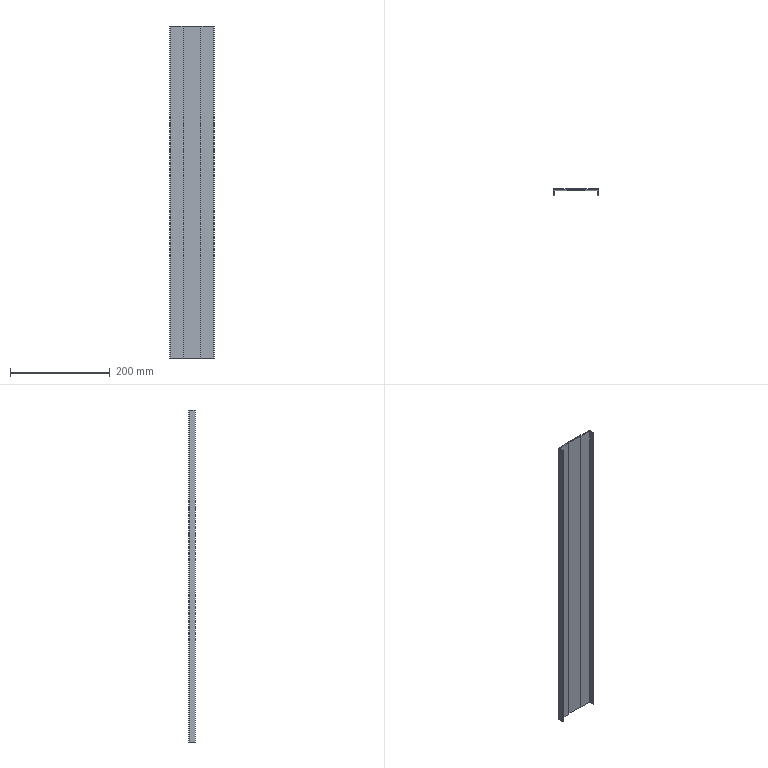Part | NX | 1 solid | 18 faces | box 89 x 13 x 666 mm | volume 147852 mm3 | plane 18
STEP:
#1=CARTESIAN_POINT('',(42.5,10.,-333.));
#2=VERTEX_POINT('',#1);
#3=CARTESIAN_POINT('',(42.5,0.,-333.));
#4=VERTEX_POINT('',#3);
#5=CARTESIAN_POINT('',(42.5,12.,-333.));
#6=DIRECTION('',(0.,-1.,0.));
#7=VECTOR('',#6,1000.);
#8=LINE('',#5,#7);
#9=EDGE_CURVE('',#2,#4,#8,.T.);
#10=ORIENTED_EDGE('',*,*,#9,.T.);
#11=CARTESIAN_POINT('',(42.5,0.,333.));
#12=VERTEX_POINT('',#11);
#13=CARTESIAN_POINT('',(42.5,0.,333.));
#14=DIRECTION('',(0.,0.,-1.));
#15=VECTOR('',#14,1000.);
#16=LINE('',#13,#15);
#17=EDGE_CURVE('',#12,#4,#16,.T.);
#18=ORIENTED_EDGE('',*,*,#17,.F.);
#19=CARTESIAN_POINT('',(42.5,10.,333.));
#20=VERTEX_POINT('',#19);
#21=CARTESIAN_POINT('',(42.5,12.,333.));
#22=DIRECTION('',(0.,-1.,0.));
#23=VECTOR('',#22,1000.);
#24=LINE('',#21,#23);
#25=EDGE_CURVE('',#20,#12,#24,.T.);
#26=ORIENTED_EDGE('',*,*,#25,.F.);
#27=CARTESIAN_POINT('',(42.5,10.,333.));
#28=DIRECTION('',(0.,0.,-1.));
#29=VECTOR('',#28,1000.);
#30=LINE('',#27,#29);
#31=EDGE_CURVE('',#20,#2,#30,.T.);
#32=ORIENTED_EDGE('',*,*,#31,.T.);
#33=EDGE_LOOP('',(#10,#18,#26,#32));
#34=FACE_BOUND('',#33,.T.);
#35=CARTESIAN_POINT('',(42.5,12.,333.));
#36=DIRECTION('',(1.,0.,0.));
#37=DIRECTION('',(0.,1.,0.));
#38=AXIS2_PLACEMENT_3D('',#35,#36,#37);
#39=PLANE('',#38);
#40=ADVANCED_FACE('',(#34),#39,.F.);
#41=CARTESIAN_POINT('',(44.5,0.,-333.));
#42=VERTEX_POINT('',#41);
#43=CARTESIAN_POINT('',(44.5,0.,-333.));
#44=DIRECTION('',(-1.,0.,0.));
#45=VECTOR('',#44,1000.);
#46=LINE('',#43,#45);
#47=EDGE_CURVE('',#42,#4,#46,.T.);
#48=ORIENTED_EDGE('',*,*,#47,.F.);
#49=CARTESIAN_POINT('',(44.5,0.,333.));
#50=VERTEX_POINT('',#49);
#51=CARTESIAN_POINT('',(44.5,0.,333.));
#52=DIRECTION('',(0.,0.,-1.));
#53=VECTOR('',#52,1000.);
#54=LINE('',#51,#53);
#55=EDGE_CURVE('',#50,#42,#54,.T.);
#56=ORIENTED_EDGE('',*,*,#55,.F.);
#57=CARTESIAN_POINT('',(44.5,0.,333.));
#58=DIRECTION('',(-1.,0.,0.));
#59=VECTOR('',#58,1000.);
#60=LINE('',#57,#59);
#61=EDGE_CURVE('',#50,#12,#60,.T.);
#62=ORIENTED_EDGE('',*,*,#61,.T.);
#63=ORIENTED_EDGE('',*,*,#17,.T.);
#64=EDGE_LOOP('',(#48,#56,#62,#63));
#65=FACE_BOUND('',#64,.T.);
#66=CARTESIAN_POINT('',(44.5,0.,333.));
#67=DIRECTION('',(0.,-1.,0.));
#68=DIRECTION('',(1.,0.,0.));
#69=AXIS2_PLACEMENT_3D('',#66,#67,#68);
#70=PLANE('',#69);
#71=ADVANCED_FACE('',(#65),#70,.T.);
#72=CARTESIAN_POINT('',(44.5,12.,-333.));
#73=VERTEX_POINT('',#72);
#74=CARTESIAN_POINT('',(44.5,12.,-333.));
#75=DIRECTION('',(0.,-1.,0.));
#76=VECTOR('',#75,1000.);
#77=LINE('',#74,#76);
#78=EDGE_CURVE('',#73,#42,#77,.T.);
#79=ORIENTED_EDGE('',*,*,#78,.F.);
#80=CARTESIAN_POINT('',(44.5,12.,333.));
#81=VERTEX_POINT('',#80);
#82=CARTESIAN_POINT('',(44.5,12.,333.));
#83=DIRECTION('',(0.,0.,-1.));
#84=VECTOR('',#83,1000.);
#85=LINE('',#82,#84);
#86=EDGE_CURVE('',#81,#73,#85,.T.);
#87=ORIENTED_EDGE('',*,*,#86,.F.);
#88=CARTESIAN_POINT('',(44.5,12.,333.));
#89=DIRECTION('',(0.,-1.,0.));
#90=VECTOR('',#89,1000.);
#91=LINE('',#88,#90);
#92=EDGE_CURVE('',#81,#50,#91,.T.);
#93=ORIENTED_EDGE('',*,*,#92,.T.);
#94=ORIENTED_EDGE('',*,*,#55,.T.);
#95=EDGE_LOOP('',(#79,#87,#93,#94));
#96=FACE_BOUND('',#95,.T.);
#97=CARTESIAN_POINT('',(44.5,12.,333.));
#98=DIRECTION('',(1.,0.,0.));
#99=DIRECTION('',(0.,1.,0.));
#100=AXIS2_PLACEMENT_3D('',#97,#98,#99);
#101=PLANE('',#100);
#102=ADVANCED_FACE('',(#96),#101,.T.);
#103=CARTESIAN_POINT('',(20.,12.,-333.));
#104=VERTEX_POINT('',#103);
#105=CARTESIAN_POINT('',(20.,12.,-333.));
#106=DIRECTION('',(1.,0.,0.));
#107=VECTOR('',#106,1000.);
#108=LINE('',#105,#107);
#109=EDGE_CURVE('',#104,#73,#108,.T.);
#110=ORIENTED_EDGE('',*,*,#109,.F.);
#111=CARTESIAN_POINT('',(20.,12.,333.));
#112=VERTEX_POINT('',#111);
#113=CARTESIAN_POINT('',(20.,12.,333.));
#114=DIRECTION('',(0.,0.,-1.));
#115=VECTOR('',#114,1000.);
#116=LINE('',#113,#115);
#117=EDGE_CURVE('',#112,#104,#116,.T.);
#118=ORIENTED_EDGE('',*,*,#117,.F.);
#119=CARTESIAN_POINT('',(20.,12.,333.));
#120=DIRECTION('',(1.,0.,0.));
#121=VECTOR('',#120,1000.);
#122=LINE('',#119,#121);
#123=EDGE_CURVE('',#112,#81,#122,.T.);
#124=ORIENTED_EDGE('',*,*,#123,.T.);
#125=ORIENTED_EDGE('',*,*,#86,.T.);
#126=EDGE_LOOP('',(#110,#118,#124,#125));
#127=FACE_BOUND('',#126,.T.);
#128=CARTESIAN_POINT('',(20.,12.,333.));
#129=DIRECTION('',(0.,1.,0.));
#130=DIRECTION('',(-1.,0.,0.));
#131=AXIS2_PLACEMENT_3D('',#128,#129,#130);
#132=PLANE('',#131);
#133=ADVANCED_FACE('',(#127),#132,.T.);
#134=CARTESIAN_POINT('',(20.,13.,-333.));
#135=VERTEX_POINT('',#134);
#136=CARTESIAN_POINT('',(20.,13.,-333.));
#137=DIRECTION('',(0.,-1.,0.));
#138=VECTOR('',#137,1000.);
#139=LINE('',#136,#138);
#140=EDGE_CURVE('',#135,#104,#139,.T.);
#141=ORIENTED_EDGE('',*,*,#140,.F.);
#142=CARTESIAN_POINT('',(20.,13.,333.));
#143=VERTEX_POINT('',#142);
#144=CARTESIAN_POINT('',(20.,13.,333.));
#145=DIRECTION('',(0.,0.,-1.));
#146=VECTOR('',#145,1000.);
#147=LINE('',#144,#146);
#148=EDGE_CURVE('',#143,#135,#147,.T.);
#149=ORIENTED_EDGE('',*,*,#148,.F.);
#150=CARTESIAN_POINT('',(20.,13.,333.));
#151=DIRECTION('',(0.,-1.,0.));
#152=VECTOR('',#151,1000.);
#153=LINE('',#150,#152);
#154=EDGE_CURVE('',#143,#112,#153,.T.);
#155=ORIENTED_EDGE('',*,*,#154,.T.);
#156=ORIENTED_EDGE('',*,*,#117,.T.);
#157=EDGE_LOOP('',(#141,#149,#155,#156));
#158=FACE_BOUND('',#157,.T.);
#159=CARTESIAN_POINT('',(20.,13.,333.));
#160=DIRECTION('',(1.,0.,0.));
#161=DIRECTION('',(0.,0.,-1.));
#162=AXIS2_PLACEMENT_3D('',#159,#160,#161);
#163=PLANE('',#162);
#164=ADVANCED_FACE('',(#158),#163,.T.);
#165=CARTESIAN_POINT('',(-20.,13.,-333.));
#166=VERTEX_POINT('',#165);
#167=CARTESIAN_POINT('',(-20.,13.,-333.));
#168=DIRECTION('',(1.,0.,0.));
#169=VECTOR('',#168,1000.);
#170=LINE('',#167,#169);
#171=EDGE_CURVE('',#166,#135,#170,.T.);
#172=ORIENTED_EDGE('',*,*,#171,.F.);
#173=CARTESIAN_POINT('',(-20.,13.,333.));
#174=VERTEX_POINT('',#173);
#175=CARTESIAN_POINT('',(-20.,13.,333.));
#176=DIRECTION('',(0.,0.,-1.));
#177=VECTOR('',#176,1000.);
#178=LINE('',#175,#177);
#179=EDGE_CURVE('',#174,#166,#178,.T.);
#180=ORIENTED_EDGE('',*,*,#179,.F.);
#181=CARTESIAN_POINT('',(-20.,13.,333.));
#182=DIRECTION('',(1.,0.,0.));
#183=VECTOR('',#182,1000.);
#184=LINE('',#181,#183);
#185=EDGE_CURVE('',#174,#143,#184,.T.);
#186=ORIENTED_EDGE('',*,*,#185,.T.);
#187=ORIENTED_EDGE('',*,*,#148,.T.);
#188=EDGE_LOOP('',(#172,#180,#186,#187));
#189=FACE_BOUND('',#188,.T.);
#190=CARTESIAN_POINT('',(-20.,13.,333.));
#191=DIRECTION('',(0.,1.,0.));
#192=DIRECTION('',(-1.,0.,0.));
#193=AXIS2_PLACEMENT_3D('',#190,#191,#192);
#194=PLANE('',#193);
#195=ADVANCED_FACE('',(#189),#194,.T.);
#196=CARTESIAN_POINT('',(-20.,12.,-333.));
#197=VERTEX_POINT('',#196);
#198=CARTESIAN_POINT('',(-20.,12.,-333.));
#199=DIRECTION('',(0.,1.,0.));
#200=VECTOR('',#199,1000.);
#201=LINE('',#198,#200);
#202=EDGE_CURVE('',#197,#166,#201,.T.);
#203=ORIENTED_EDGE('',*,*,#202,.F.);
#204=CARTESIAN_POINT('',(-20.,12.,333.));
#205=VERTEX_POINT('',#204);
#206=CARTESIAN_POINT('',(-20.,12.,333.));
#207=DIRECTION('',(0.,0.,-1.));
#208=VECTOR('',#207,1000.);
#209=LINE('',#206,#208);
#210=EDGE_CURVE('',#205,#197,#209,.T.);
#211=ORIENTED_EDGE('',*,*,#210,.F.);
#212=CARTESIAN_POINT('',(-20.,12.,333.));
#213=DIRECTION('',(0.,1.,0.));
#214=VECTOR('',#213,1000.);
#215=LINE('',#212,#214);
#216=EDGE_CURVE('',#205,#174,#215,.T.);
#217=ORIENTED_EDGE('',*,*,#216,.T.);
#218=ORIENTED_EDGE('',*,*,#179,.T.);
#219=EDGE_LOOP('',(#203,#211,#217,#218));
#220=FACE_BOUND('',#219,.T.);
#221=CARTESIAN_POINT('',(-20.,12.,333.));
#222=DIRECTION('',(-1.,0.,0.));
#223=DIRECTION('',(0.,0.,1.));
#224=AXIS2_PLACEMENT_3D('',#221,#222,#223);
#225=PLANE('',#224);
#226=ADVANCED_FACE('',(#220),#225,.T.);
#227=CARTESIAN_POINT('',(-44.5,12.,-333.));
#228=VERTEX_POINT('',#227);
#229=CARTESIAN_POINT('',(-44.5,12.,-333.));
#230=DIRECTION('',(1.,0.,0.));
#231=VECTOR('',#230,1000.);
#232=LINE('',#229,#231);
#233=EDGE_CURVE('',#228,#197,#232,.T.);
#234=ORIENTED_EDGE('',*,*,#233,.F.);
#235=CARTESIAN_POINT('',(-44.5,12.,333.));
#236=VERTEX_POINT('',#235);
#237=CARTESIAN_POINT('',(-44.5,12.,333.));
#238=DIRECTION('',(0.,0.,-1.));
#239=VECTOR('',#238,1000.);
#240=LINE('',#237,#239);
#241=EDGE_CURVE('',#236,#228,#240,.T.);
#242=ORIENTED_EDGE('',*,*,#241,.F.);
#243=CARTESIAN_POINT('',(-44.5,12.,333.));
#244=DIRECTION('',(1.,0.,0.));
#245=VECTOR('',#244,1000.);
#246=LINE('',#243,#245);
#247=EDGE_CURVE('',#236,#205,#246,.T.);
#248=ORIENTED_EDGE('',*,*,#247,.T.);
#249=ORIENTED_EDGE('',*,*,#210,.T.);
#250=EDGE_LOOP('',(#234,#242,#248,#249));
#251=FACE_BOUND('',#250,.T.);
#252=CARTESIAN_POINT('',(-44.5,12.,333.));
#253=DIRECTION('',(0.,1.,0.));
#254=DIRECTION('',(0.,0.,1.));
#255=AXIS2_PLACEMENT_3D('',#252,#253,#254);
#256=PLANE('',#255);
#257=ADVANCED_FACE('',(#251),#256,.T.);
#258=CARTESIAN_POINT('',(-44.5,0.,-333.));
#259=VERTEX_POINT('',#258);
#260=CARTESIAN_POINT('',(-44.5,0.,-333.));
#261=DIRECTION('',(0.,1.,0.));
#262=VECTOR('',#261,1000.);
#263=LINE('',#260,#262);
#264=EDGE_CURVE('',#259,#228,#263,.T.);
#265=ORIENTED_EDGE('',*,*,#264,.F.);
#266=CARTESIAN_POINT('',(-44.5,0.,333.));
#267=VERTEX_POINT('',#266);
#268=CARTESIAN_POINT('',(-44.5,0.,333.));
#269=DIRECTION('',(0.,0.,-1.));
#270=VECTOR('',#269,1000.);
#271=LINE('',#268,#270);
#272=EDGE_CURVE('',#267,#259,#271,.T.);
#273=ORIENTED_EDGE('',*,*,#272,.F.);
#274=CARTESIAN_POINT('',(-44.5,0.,333.));
#275=DIRECTION('',(0.,1.,0.));
#276=VECTOR('',#275,1000.);
#277=LINE('',#274,#276);
#278=EDGE_CURVE('',#267,#236,#277,.T.);
#279=ORIENTED_EDGE('',*,*,#278,.T.);
#280=ORIENTED_EDGE('',*,*,#241,.T.);
#281=EDGE_LOOP('',(#265,#273,#279,#280));
#282=FACE_BOUND('',#281,.T.);
#283=CARTESIAN_POINT('',(-44.5,0.,333.));
#284=DIRECTION('',(-1.,0.,0.));
#285=DIRECTION('',(0.,0.,1.));
#286=AXIS2_PLACEMENT_3D('',#283,#284,#285);
#287=PLANE('',#286);
#288=ADVANCED_FACE('',(#282),#287,.T.);
#289=CARTESIAN_POINT('',(-42.5,0.,-333.));
#290=VERTEX_POINT('',#289);
#291=CARTESIAN_POINT('',(-42.5,0.,-333.));
#292=DIRECTION('',(-1.,0.,0.));
#293=VECTOR('',#292,1000.);
#294=LINE('',#291,#293);
#295=EDGE_CURVE('',#290,#259,#294,.T.);
#296=ORIENTED_EDGE('',*,*,#295,.F.);
#297=CARTESIAN_POINT('',(-42.5,0.,333.));
#298=VERTEX_POINT('',#297);
#299=CARTESIAN_POINT('',(-42.5,0.,333.));
#300=DIRECTION('',(0.,0.,-1.));
#301=VECTOR('',#300,1000.);
#302=LINE('',#299,#301);
#303=EDGE_CURVE('',#298,#290,#302,.T.);
#304=ORIENTED_EDGE('',*,*,#303,.F.);
#305=CARTESIAN_POINT('',(-42.5,0.,333.));
#306=DIRECTION('',(-1.,0.,0.));
#307=VECTOR('',#306,1000.);
#308=LINE('',#305,#307);
#309=EDGE_CURVE('',#298,#267,#308,.T.);
#310=ORIENTED_EDGE('',*,*,#309,.T.);
#311=ORIENTED_EDGE('',*,*,#272,.T.);
#312=EDGE_LOOP('',(#296,#304,#310,#311));
#313=FACE_BOUND('',#312,.T.);
#314=CARTESIAN_POINT('',(-42.5,0.,333.));
#315=DIRECTION('',(0.,-1.,0.));
#316=DIRECTION('',(0.,0.,-1.));
#317=AXIS2_PLACEMENT_3D('',#314,#315,#316);
#318=PLANE('',#317);
#319=ADVANCED_FACE('',(#313),#318,.T.);
#320=CARTESIAN_POINT('',(-42.5,10.,-333.));
#321=VERTEX_POINT('',#320);
#322=CARTESIAN_POINT('',(-42.5,0.,-333.));
#323=DIRECTION('',(0.,1.,0.));
#324=VECTOR('',#323,1000.);
#325=LINE('',#322,#324);
#326=EDGE_CURVE('',#290,#321,#325,.T.);
#327=ORIENTED_EDGE('',*,*,#326,.T.);
#328=CARTESIAN_POINT('',(-42.5,10.,333.));
#329=VERTEX_POINT('',#328);
#330=CARTESIAN_POINT('',(-42.5,10.,333.));
#331=DIRECTION('',(0.,0.,-1.));
#332=VECTOR('',#331,1000.);
#333=LINE('',#330,#332);
#334=EDGE_CURVE('',#329,#321,#333,.T.);
#335=ORIENTED_EDGE('',*,*,#334,.F.);
#336=CARTESIAN_POINT('',(-42.5,0.,333.));
#337=DIRECTION('',(0.,1.,0.));
#338=VECTOR('',#337,1000.);
#339=LINE('',#336,#338);
#340=EDGE_CURVE('',#298,#329,#339,.T.);
#341=ORIENTED_EDGE('',*,*,#340,.F.);
#342=ORIENTED_EDGE('',*,*,#303,.T.);
#343=EDGE_LOOP('',(#327,#335,#341,#342));
#344=FACE_BOUND('',#343,.T.);
#345=CARTESIAN_POINT('',(-42.5,0.,333.));
#346=DIRECTION('',(-1.,0.,0.));
#347=DIRECTION('',(0.,0.,1.));
#348=AXIS2_PLACEMENT_3D('',#345,#346,#347);
#349=PLANE('',#348);
#350=ADVANCED_FACE('',(#344),#349,.F.);
#351=CARTESIAN_POINT('',(-18.,10.,-333.));
#352=VERTEX_POINT('',#351);
#353=CARTESIAN_POINT('',(-44.5,10.,-333.));
#354=DIRECTION('',(1.,0.,0.));
#355=VECTOR('',#354,1000.);
#356=LINE('',#353,#355);
#357=EDGE_CURVE('',#321,#352,#356,.T.);
#358=ORIENTED_EDGE('',*,*,#357,.T.);
#359=CARTESIAN_POINT('',(-18.,10.,333.));
#360=VERTEX_POINT('',#359);
#361=CARTESIAN_POINT('',(-18.,10.,333.));
#362=DIRECTION('',(0.,0.,-1.));
#363=VECTOR('',#362,1000.);
#364=LINE('',#361,#363);
#365=EDGE_CURVE('',#360,#352,#364,.T.);
#366=ORIENTED_EDGE('',*,*,#365,.F.);
#367=CARTESIAN_POINT('',(-44.5,10.,333.));
#368=DIRECTION('',(1.,0.,0.));
#369=VECTOR('',#368,1000.);
#370=LINE('',#367,#369);
#371=EDGE_CURVE('',#329,#360,#370,.T.);
#372=ORIENTED_EDGE('',*,*,#371,.F.);
#373=ORIENTED_EDGE('',*,*,#334,.T.);
#374=EDGE_LOOP('',(#358,#366,#372,#373));
#375=FACE_BOUND('',#374,.T.);
#376=CARTESIAN_POINT('',(-44.5,10.,333.));
#377=DIRECTION('',(0.,1.,0.));
#378=DIRECTION('',(0.,0.,1.));
#379=AXIS2_PLACEMENT_3D('',#376,#377,#378);
#380=PLANE('',#379);
#381=ADVANCED_FACE('',(#375),#380,.F.);
#382=CARTESIAN_POINT('',(-18.,11.,-333.));
#383=VERTEX_POINT('',#382);
#384=CARTESIAN_POINT('',(-18.,12.,-333.));
#385=DIRECTION('',(0.,1.,0.));
#386=VECTOR('',#385,1000.);
#387=LINE('',#384,#386);
#388=EDGE_CURVE('',#352,#383,#387,.T.);
#389=ORIENTED_EDGE('',*,*,#388,.T.);
#390=CARTESIAN_POINT('',(-18.,11.,333.));
#391=VERTEX_POINT('',#390);
#392=CARTESIAN_POINT('',(-18.,11.,333.));
#393=DIRECTION('',(0.,0.,-1.));
#394=VECTOR('',#393,1000.);
#395=LINE('',#392,#394);
#396=EDGE_CURVE('',#391,#383,#395,.T.);
#397=ORIENTED_EDGE('',*,*,#396,.F.);
#398=CARTESIAN_POINT('',(-18.,12.,333.));
#399=DIRECTION('',(0.,1.,0.));
#400=VECTOR('',#399,1000.);
#401=LINE('',#398,#400);
#402=EDGE_CURVE('',#360,#391,#401,.T.);
#403=ORIENTED_EDGE('',*,*,#402,.F.);
#404=ORIENTED_EDGE('',*,*,#365,.T.);
#405=EDGE_LOOP('',(#389,#397,#403,#404));
#406=FACE_BOUND('',#405,.T.);
#407=CARTESIAN_POINT('',(-18.,12.,333.));
#408=DIRECTION('',(-1.,0.,0.));
#409=DIRECTION('',(0.,0.,1.));
#410=AXIS2_PLACEMENT_3D('',#407,#408,#409);
#411=PLANE('',#410);
#412=ADVANCED_FACE('',(#406),#411,.F.);
#413=CARTESIAN_POINT('',(18.,11.,-333.));
#414=VERTEX_POINT('',#413);
#415=CARTESIAN_POINT('',(-20.,11.,-333.));
#416=DIRECTION('',(1.,0.,0.));
#417=VECTOR('',#416,1000.);
#418=LINE('',#415,#417);
#419=EDGE_CURVE('',#383,#414,#418,.T.);
#420=ORIENTED_EDGE('',*,*,#419,.T.);
#421=CARTESIAN_POINT('',(18.,11.,333.));
#422=VERTEX_POINT('',#421);
#423=CARTESIAN_POINT('',(18.,11.,333.));
#424=DIRECTION('',(0.,0.,-1.));
#425=VECTOR('',#424,1000.);
#426=LINE('',#423,#425);
#427=EDGE_CURVE('',#422,#414,#426,.T.);
#428=ORIENTED_EDGE('',*,*,#427,.F.);
#429=CARTESIAN_POINT('',(-20.,11.,333.));
#430=DIRECTION('',(1.,0.,0.));
#431=VECTOR('',#430,1000.);
#432=LINE('',#429,#431);
#433=EDGE_CURVE('',#391,#422,#432,.T.);
#434=ORIENTED_EDGE('',*,*,#433,.F.);
#435=ORIENTED_EDGE('',*,*,#396,.T.);
#436=EDGE_LOOP('',(#420,#428,#434,#435));
#437=FACE_BOUND('',#436,.T.);
#438=CARTESIAN_POINT('',(-20.,11.,333.));
#439=DIRECTION('',(0.,1.,0.));
#440=DIRECTION('',(-1.,0.,0.));
#441=AXIS2_PLACEMENT_3D('',#438,#439,#440);
#442=PLANE('',#441);
#443=ADVANCED_FACE('',(#437),#442,.F.);
#444=CARTESIAN_POINT('',(18.,10.,-333.));
#445=VERTEX_POINT('',#444);
#446=CARTESIAN_POINT('',(18.,13.,-333.));
#447=DIRECTION('',(0.,1.,0.));
#448=VECTOR('',#447,1000.);
#449=LINE('',#446,#448);
#450=EDGE_CURVE('',#414,#445,#449,.F.);
#451=ORIENTED_EDGE('',*,*,#450,.T.);
#452=CARTESIAN_POINT('',(18.,10.,333.));
#453=VERTEX_POINT('',#452);
#454=CARTESIAN_POINT('',(18.,10.,333.));
#455=DIRECTION('',(0.,0.,-1.));
#456=VECTOR('',#455,1000.);
#457=LINE('',#454,#456);
#458=EDGE_CURVE('',#453,#445,#457,.T.);
#459=ORIENTED_EDGE('',*,*,#458,.F.);
#460=CARTESIAN_POINT('',(18.,13.,333.));
#461=DIRECTION('',(0.,1.,0.));
#462=VECTOR('',#461,1000.);
#463=LINE('',#460,#462);
#464=EDGE_CURVE('',#422,#453,#463,.F.);
#465=ORIENTED_EDGE('',*,*,#464,.F.);
#466=ORIENTED_EDGE('',*,*,#427,.T.);
#467=EDGE_LOOP('',(#451,#459,#465,#466));
#468=FACE_BOUND('',#467,.T.);
#469=CARTESIAN_POINT('',(18.,13.,333.));
#470=DIRECTION('',(1.,0.,0.));
#471=DIRECTION('',(0.,0.,-1.));
#472=AXIS2_PLACEMENT_3D('',#469,#470,#471);
#473=PLANE('',#472);
#474=ADVANCED_FACE('',(#468),#473,.F.);
#475=CARTESIAN_POINT('',(20.,10.,-333.));
#476=DIRECTION('',(1.,0.,0.));
#477=VECTOR('',#476,1000.);
#478=LINE('',#475,#477);
#479=EDGE_CURVE('',#445,#2,#478,.T.);
#480=ORIENTED_EDGE('',*,*,#479,.T.);
#481=ORIENTED_EDGE('',*,*,#31,.F.);
#482=CARTESIAN_POINT('',(20.,10.,333.));
#483=DIRECTION('',(1.,0.,0.));
#484=VECTOR('',#483,1000.);
#485=LINE('',#482,#484);
#486=EDGE_CURVE('',#453,#20,#485,.T.);
#487=ORIENTED_EDGE('',*,*,#486,.F.);
#488=ORIENTED_EDGE('',*,*,#458,.T.);
#489=EDGE_LOOP('',(#480,#481,#487,#488));
#490=FACE_BOUND('',#489,.T.);
#491=CARTESIAN_POINT('',(20.,10.,333.));
#492=DIRECTION('',(0.,1.,0.));
#493=DIRECTION('',(-1.,0.,0.));
#494=AXIS2_PLACEMENT_3D('',#491,#492,#493);
#495=PLANE('',#494);
#496=ADVANCED_FACE('',(#490),#495,.F.);
#497=ORIENTED_EDGE('',*,*,#25,.T.);
#498=ORIENTED_EDGE('',*,*,#61,.F.);
#499=ORIENTED_EDGE('',*,*,#92,.F.);
#500=ORIENTED_EDGE('',*,*,#123,.F.);
#501=ORIENTED_EDGE('',*,*,#154,.F.);
#502=ORIENTED_EDGE('',*,*,#185,.F.);
#503=ORIENTED_EDGE('',*,*,#216,.F.);
#504=ORIENTED_EDGE('',*,*,#247,.F.);
#505=ORIENTED_EDGE('',*,*,#278,.F.);
#506=ORIENTED_EDGE('',*,*,#309,.F.);
#507=ORIENTED_EDGE('',*,*,#340,.T.);
#508=ORIENTED_EDGE('',*,*,#371,.T.);
#509=ORIENTED_EDGE('',*,*,#402,.T.);
#510=ORIENTED_EDGE('',*,*,#433,.T.);
#511=ORIENTED_EDGE('',*,*,#464,.T.);
#512=ORIENTED_EDGE('',*,*,#486,.T.);
#513=EDGE_LOOP('',(#497,#498,#499,#500,#501,#502,#503,#504,#505,#506,#507,#508,#509,#510,#511,#512));
#514=FACE_BOUND('',#513,.T.);
#515=CARTESIAN_POINT('',(0.,0.,333.));
#516=DIRECTION('',(0.,0.,-1.));
#517=DIRECTION('',(-1.,0.,0.));
#518=AXIS2_PLACEMENT_3D('',#515,#516,#517);
#519=PLANE('',#518);
#520=ADVANCED_FACE('',(#514),#519,.F.);
#521=ORIENTED_EDGE('',*,*,#9,.F.);
#522=ORIENTED_EDGE('',*,*,#479,.F.);
#523=ORIENTED_EDGE('',*,*,#450,.F.);
#524=ORIENTED_EDGE('',*,*,#419,.F.);
#525=ORIENTED_EDGE('',*,*,#388,.F.);
#526=ORIENTED_EDGE('',*,*,#357,.F.);
#527=ORIENTED_EDGE('',*,*,#326,.F.);
#528=ORIENTED_EDGE('',*,*,#295,.T.);
#529=ORIENTED_EDGE('',*,*,#264,.T.);
#530=ORIENTED_EDGE('',*,*,#233,.T.);
#531=ORIENTED_EDGE('',*,*,#202,.T.);
#532=ORIENTED_EDGE('',*,*,#171,.T.);
#533=ORIENTED_EDGE('',*,*,#140,.T.);
#534=ORIENTED_EDGE('',*,*,#109,.T.);
#535=ORIENTED_EDGE('',*,*,#78,.T.);
#536=ORIENTED_EDGE('',*,*,#47,.T.);
#537=EDGE_LOOP('',(#521,#522,#523,#524,#525,#526,#527,#528,#529,#530,#531,#532,#533,#534,#535,#536));
#538=FACE_BOUND('',#537,.T.);
#539=CARTESIAN_POINT('',(0.,0.,-333.));
#540=DIRECTION('',(0.,0.,-1.));
#541=DIRECTION('',(-1.,0.,0.));
#542=AXIS2_PLACEMENT_3D('',#539,#540,#541);
#543=PLANE('',#542);
#544=ADVANCED_FACE('',(#538),#543,.T.);
#545=CLOSED_SHELL('',(#40,#71,#102,#133,#164,#195,#226,#257,#288,#319,#350,#381,#412,#443,#474,#496,#520,#544));
#546=MANIFOLD_SOLID_BREP('',#545);
#547=(LENGTH_UNIT()NAMED_UNIT(*)SI_UNIT(.MILLI.,.METRE.));
#548=UNCERTAINTY_MEASURE_WITH_UNIT(LENGTH_MEASURE(0.00001),#547,'','');
#549=(NAMED_UNIT(*)PLANE_ANGLE_UNIT()SI_UNIT($,.RADIAN.));
#550=(NAMED_UNIT(*)SI_UNIT($,.STERADIAN.)SOLID_ANGLE_UNIT());
#551=(GEOMETRIC_REPRESENTATION_CONTEXT(3)GLOBAL_UNCERTAINTY_ASSIGNED_CONTEXT((#548))GLOBAL_UNIT_ASSIGNED_CONTEXT((#547,#549,#550))REPRESENTATION_CONTEXT('',''));
#552=ADVANCED_BREP_SHAPE_REPRESENTATION('',(#546),#551);